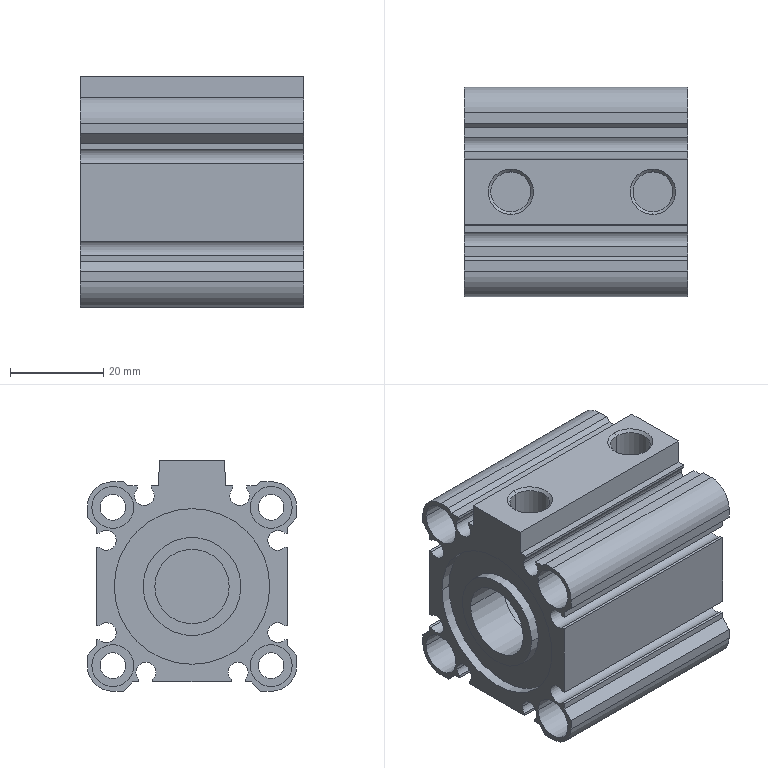Part | STEP file | 25A-CDQ2B32-15DZ-M9BWSDPC-Part-2-4 | 1 solid | 126 faces | box 48 x 45 x 49.5 mm | volume 58108 mm3 | plane 64 | cylinder 58 | cone 4 | commonest cylinder face diameters 4.26 x18 9 x16 5.5 x8 8.566 x4 11 x4 16 x2